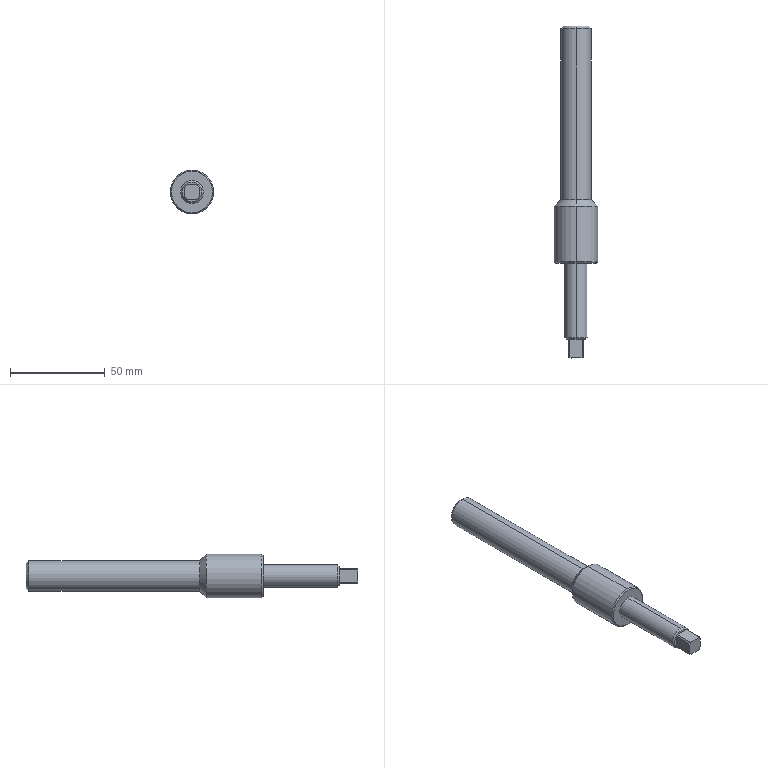Part | SolidWorks | features BaseBody 1 | 1 solid | 33 faces | box 23 x 175 x 23 mm | volume 36998 mm3 | cone 12 | plane 11 | cylinder 10 | commonest cylinder face diameters 10.5 x4 12 x2 16 x2 23 x2
STEP:
#1=CARTESIAN_POINT('',(0.,83.5,8.));
#2=VERTEX_POINT('',#1);
#3=CARTESIAN_POINT('',(0.,83.5,-8.));
#4=VERTEX_POINT('',#3);
#5=CARTESIAN_POINT('',(0.,83.5,0.));
#6=DIRECTION('',(0.,1.,0.));
#7=DIRECTION('',(0.,0.,1.));
#8=AXIS2_PLACEMENT_3D('',#5,#6,#7);
#9=CIRCLE('',#8,8.);
#10=EDGE_CURVE('',#2,#4,#9,.T.);
#11=ORIENTED_EDGE('',*,*,#10,.T.);
#12=CARTESIAN_POINT('',(0.,173.5,-8.));
#13=VERTEX_POINT('',#12);
#14=CARTESIAN_POINT('',(0.,175.,-8.));
#15=DIRECTION('',(0.,1.,0.));
#16=VECTOR('',#15,1000.);
#17=LINE('',#14,#16);
#18=EDGE_CURVE('',#4,#13,#17,.T.);
#19=ORIENTED_EDGE('',*,*,#18,.T.);
#20=CARTESIAN_POINT('',(0.,173.5,8.));
#21=VERTEX_POINT('',#20);
#22=CARTESIAN_POINT('',(0.,173.5,0.));
#23=DIRECTION('',(0.,-1.,0.));
#24=DIRECTION('',(0.,0.,1.));
#25=AXIS2_PLACEMENT_3D('',#22,#23,#24);
#26=CIRCLE('',#25,8.);
#27=EDGE_CURVE('',#13,#21,#26,.T.);
#28=ORIENTED_EDGE('',*,*,#27,.T.);
#29=CARTESIAN_POINT('',(0.,175.,8.));
#30=DIRECTION('',(0.,1.,0.));
#31=VECTOR('',#30,1000.);
#32=LINE('',#29,#31);
#33=EDGE_CURVE('',#2,#21,#32,.T.);
#34=ORIENTED_EDGE('',*,*,#33,.F.);
#35=EDGE_LOOP('',(#11,#19,#28,#34));
#36=FACE_OUTER_BOUND('',#35,.T.);
#37=CARTESIAN_POINT('',(0.,175.,0.));
#38=DIRECTION('',(0.,1.,0.));
#39=DIRECTION('',(0.,0.,1.));
#40=AXIS2_PLACEMENT_3D('',#37,#38,#39);
#41=CYLINDRICAL_SURFACE('',#40,8.);
#42=ADVANCED_FACE('',(#36),#41,.T.);
#43=CARTESIAN_POINT('',(0.,175.,-6.5));
#44=VERTEX_POINT('',#43);
#45=CARTESIAN_POINT('',(0.,175.,6.5));
#46=VERTEX_POINT('',#45);
#47=CARTESIAN_POINT('',(0.,175.,0.));
#48=DIRECTION('',(0.,-1.,0.));
#49=DIRECTION('',(0.,0.,-1.));
#50=AXIS2_PLACEMENT_3D('',#47,#48,#49);
#51=CIRCLE('',#50,6.5);
#52=EDGE_CURVE('',#44,#46,#51,.T.);
#53=ORIENTED_EDGE('',*,*,#52,.T.);
#54=CARTESIAN_POINT('',(0.,173.5,8.));
#55=DIRECTION('',(0.,-0.7071,0.7071));
#56=VECTOR('',#55,1000.);
#57=LINE('',#54,#56);
#58=EDGE_CURVE('',#46,#21,#57,.T.);
#59=ORIENTED_EDGE('',*,*,#58,.T.);
#60=ORIENTED_EDGE('',*,*,#27,.F.);
#61=CARTESIAN_POINT('',(0.,173.5,-8.));
#62=DIRECTION('',(0.,-0.7071,-0.7071));
#63=VECTOR('',#62,1000.);
#64=LINE('',#61,#63);
#65=EDGE_CURVE('',#44,#13,#64,.T.);
#66=ORIENTED_EDGE('',*,*,#65,.F.);
#67=EDGE_LOOP('',(#53,#59,#60,#66));
#68=FACE_OUTER_BOUND('',#67,.T.);
#69=CARTESIAN_POINT('',(0.,173.5,0.));
#70=DIRECTION('',(0.,-1.,0.));
#71=DIRECTION('',(0.,0.,-1.));
#72=AXIS2_PLACEMENT_3D('',#69,#70,#71);
#73=CONICAL_SURFACE('',#72,8.,0.7854);
#74=ADVANCED_FACE('',(#68),#73,.T.);
#75=ORIENTED_EDGE('',*,*,#10,.F.);
#76=CARTESIAN_POINT('',(0.,80.,11.5));
#77=VERTEX_POINT('',#76);
#78=CARTESIAN_POINT('',(0.,80.,11.5));
#79=DIRECTION('',(0.,-0.7071,0.7071));
#80=VECTOR('',#79,1000.);
#81=LINE('',#78,#80);
#82=EDGE_CURVE('',#2,#77,#81,.T.);
#83=ORIENTED_EDGE('',*,*,#82,.T.);
#84=CARTESIAN_POINT('',(0.,80.,-11.5));
#85=VERTEX_POINT('',#84);
#86=CARTESIAN_POINT('',(0.,80.,0.));
#87=DIRECTION('',(0.,1.,0.));
#88=DIRECTION('',(1.,0.,0.));
#89=AXIS2_PLACEMENT_3D('',#86,#87,#88);
#90=CIRCLE('',#89,11.5);
#91=EDGE_CURVE('',#77,#85,#90,.T.);
#92=ORIENTED_EDGE('',*,*,#91,.T.);
#93=CARTESIAN_POINT('',(0.,80.,-11.5));
#94=DIRECTION('',(0.,-0.7071,-0.7071));
#95=VECTOR('',#94,1000.);
#96=LINE('',#93,#95);
#97=EDGE_CURVE('',#4,#85,#96,.T.);
#98=ORIENTED_EDGE('',*,*,#97,.F.);
#99=EDGE_LOOP('',(#75,#83,#92,#98));
#100=FACE_OUTER_BOUND('',#99,.T.);
#101=CARTESIAN_POINT('',(0.,80.,0.));
#102=DIRECTION('',(0.,-1.,0.));
#103=DIRECTION('',(0.,0.,-1.));
#104=AXIS2_PLACEMENT_3D('',#101,#102,#103);
#105=CONICAL_SURFACE('',#104,11.5,0.7854);
#106=ADVANCED_FACE('',(#100),#105,.T.);
#107=CARTESIAN_POINT('',(0.,50.6,11.5));
#108=VERTEX_POINT('',#107);
#109=CARTESIAN_POINT('',(0.,50.6,-11.5));
#110=VERTEX_POINT('',#109);
#111=CARTESIAN_POINT('',(0.,50.6,0.));
#112=DIRECTION('',(0.,1.,0.));
#113=DIRECTION('',(0.,0.,1.));
#114=AXIS2_PLACEMENT_3D('',#111,#112,#113);
#115=CIRCLE('',#114,11.5);
#116=EDGE_CURVE('',#108,#110,#115,.T.);
#117=ORIENTED_EDGE('',*,*,#116,.T.);
#118=CARTESIAN_POINT('',(0.,175.,-11.5));
#119=DIRECTION('',(0.,1.,0.));
#120=VECTOR('',#119,1000.);
#121=LINE('',#118,#120);
#122=EDGE_CURVE('',#110,#85,#121,.T.);
#123=ORIENTED_EDGE('',*,*,#122,.T.);
#124=ORIENTED_EDGE('',*,*,#91,.F.);
#125=CARTESIAN_POINT('',(0.,175.,11.5));
#126=DIRECTION('',(0.,1.,0.));
#127=VECTOR('',#126,1000.);
#128=LINE('',#125,#127);
#129=EDGE_CURVE('',#108,#77,#128,.T.);
#130=ORIENTED_EDGE('',*,*,#129,.F.);
#131=EDGE_LOOP('',(#117,#123,#124,#130));
#132=FACE_OUTER_BOUND('',#131,.T.);
#133=CARTESIAN_POINT('',(0.,175.,0.));
#134=DIRECTION('',(0.,1.,0.));
#135=DIRECTION('',(0.,0.,1.));
#136=AXIS2_PLACEMENT_3D('',#133,#134,#135);
#137=CYLINDRICAL_SURFACE('',#136,11.5);
#138=ADVANCED_FACE('',(#132),#137,.T.);
#139=CARTESIAN_POINT('',(0.,50.,10.9));
#140=VERTEX_POINT('',#139);
#141=CARTESIAN_POINT('',(0.,50.,-10.9));
#142=VERTEX_POINT('',#141);
#143=CARTESIAN_POINT('',(0.,50.,0.));
#144=DIRECTION('',(0.,1.,0.));
#145=DIRECTION('',(0.,0.,1.));
#146=AXIS2_PLACEMENT_3D('',#143,#144,#145);
#147=CIRCLE('',#146,10.9);
#148=EDGE_CURVE('',#140,#142,#147,.T.);
#149=ORIENTED_EDGE('',*,*,#148,.T.);
#150=CARTESIAN_POINT('',(0.,50.6,-11.5));
#151=DIRECTION('',(0.,0.7071,-0.7071));
#152=VECTOR('',#151,1000.);
#153=LINE('',#150,#152);
#154=EDGE_CURVE('',#142,#110,#153,.T.);
#155=ORIENTED_EDGE('',*,*,#154,.T.);
#156=ORIENTED_EDGE('',*,*,#116,.F.);
#157=CARTESIAN_POINT('',(0.,50.6,11.5));
#158=DIRECTION('',(0.,0.7071,0.7071));
#159=VECTOR('',#158,1000.);
#160=LINE('',#157,#159);
#161=EDGE_CURVE('',#140,#108,#160,.T.);
#162=ORIENTED_EDGE('',*,*,#161,.F.);
#163=EDGE_LOOP('',(#149,#155,#156,#162));
#164=FACE_OUTER_BOUND('',#163,.T.);
#165=CARTESIAN_POINT('',(0.,50.6,0.));
#166=DIRECTION('',(0.,1.,0.));
#167=DIRECTION('',(0.,0.,1.));
#168=AXIS2_PLACEMENT_3D('',#165,#166,#167);
#169=CONICAL_SURFACE('',#168,11.5,0.7854);
#170=ADVANCED_FACE('',(#164),#169,.T.);
#171=CARTESIAN_POINT('',(0.,10.75,6.));
#172=VERTEX_POINT('',#171);
#173=CARTESIAN_POINT('',(0.,10.75,-6.));
#174=VERTEX_POINT('',#173);
#175=CARTESIAN_POINT('',(0.,10.75,0.));
#176=DIRECTION('',(0.,1.,0.));
#177=DIRECTION('',(0.,0.,1.));
#178=AXIS2_PLACEMENT_3D('',#175,#176,#177);
#179=CIRCLE('',#178,6.);
#180=EDGE_CURVE('',#172,#174,#179,.T.);
#181=ORIENTED_EDGE('',*,*,#180,.T.);
#182=CARTESIAN_POINT('',(0.,50.,-6.));
#183=VERTEX_POINT('',#182);
#184=CARTESIAN_POINT('',(0.,175.,-6.));
#185=DIRECTION('',(0.,1.,0.));
#186=VECTOR('',#185,1000.);
#187=LINE('',#184,#186);
#188=EDGE_CURVE('',#174,#183,#187,.T.);
#189=ORIENTED_EDGE('',*,*,#188,.T.);
#190=CARTESIAN_POINT('',(0.,50.,6.));
#191=VERTEX_POINT('',#190);
#192=CARTESIAN_POINT('',(0.,50.,0.));
#193=DIRECTION('',(0.,1.,0.));
#194=DIRECTION('',(0.,0.,1.));
#195=AXIS2_PLACEMENT_3D('',#192,#193,#194);
#196=CIRCLE('',#195,6.);
#197=EDGE_CURVE('',#191,#183,#196,.T.);
#198=ORIENTED_EDGE('',*,*,#197,.F.);
#199=CARTESIAN_POINT('',(0.,175.,6.));
#200=DIRECTION('',(0.,1.,0.));
#201=VECTOR('',#200,1000.);
#202=LINE('',#199,#201);
#203=EDGE_CURVE('',#172,#191,#202,.T.);
#204=ORIENTED_EDGE('',*,*,#203,.F.);
#205=EDGE_LOOP('',(#181,#189,#198,#204));
#206=FACE_OUTER_BOUND('',#205,.T.);
#207=CARTESIAN_POINT('',(0.,175.,0.));
#208=DIRECTION('',(0.,1.,0.));
#209=DIRECTION('',(0.,0.,1.));
#210=AXIS2_PLACEMENT_3D('',#207,#208,#209);
#211=CYLINDRICAL_SURFACE('',#210,6.);
#212=ADVANCED_FACE('',(#206),#211,.T.);
#213=CARTESIAN_POINT('',(3.4,10.,-4.));
#214=VERTEX_POINT('',#213);
#215=CARTESIAN_POINT('',(0.,10.,-5.25));
#216=VERTEX_POINT('',#215);
#217=CARTESIAN_POINT('',(0.,10.,0.));
#218=DIRECTION('',(0.,1.,0.));
#219=DIRECTION('',(0.,0.,1.));
#220=AXIS2_PLACEMENT_3D('',#217,#218,#219);
#221=CIRCLE('',#220,5.25);
#222=EDGE_CURVE('',#214,#216,#221,.T.);
#223=ORIENTED_EDGE('',*,*,#222,.T.);
#224=CARTESIAN_POINT('',(0.,10.75,-6.));
#225=DIRECTION('',(0.,0.7071,-0.7071));
#226=VECTOR('',#225,1000.);
#227=LINE('',#224,#226);
#228=EDGE_CURVE('',#216,#174,#227,.T.);
#229=ORIENTED_EDGE('',*,*,#228,.T.);
#230=ORIENTED_EDGE('',*,*,#180,.F.);
#231=CARTESIAN_POINT('',(0.,10.,5.25));
#232=VERTEX_POINT('',#231);
#233=CARTESIAN_POINT('',(0.,10.75,6.));
#234=DIRECTION('',(0.,0.7071,0.7071));
#235=VECTOR('',#234,1000.);
#236=LINE('',#233,#235);
#237=EDGE_CURVE('',#232,#172,#236,.T.);
#238=ORIENTED_EDGE('',*,*,#237,.F.);
#239=CARTESIAN_POINT('',(3.4,10.,4.));
#240=VERTEX_POINT('',#239);
#241=CARTESIAN_POINT('',(0.,10.,0.));
#242=DIRECTION('',(0.,1.,0.));
#243=DIRECTION('',(0.,0.,1.));
#244=AXIS2_PLACEMENT_3D('',#241,#242,#243);
#245=CIRCLE('',#244,5.25);
#246=EDGE_CURVE('',#232,#240,#245,.T.);
#247=ORIENTED_EDGE('',*,*,#246,.T.);
#248=CARTESIAN_POINT('',(4.,10.,3.4));
#249=VERTEX_POINT('',#248);
#250=CARTESIAN_POINT('',(0.,10.,0.));
#251=DIRECTION('',(0.,-1.,0.));
#252=DIRECTION('',(0.,0.,1.));
#253=AXIS2_PLACEMENT_3D('',#250,#251,#252);
#254=CIRCLE('',#253,5.25);
#255=EDGE_CURVE('',#249,#240,#254,.T.);
#256=ORIENTED_EDGE('',*,*,#255,.F.);
#257=CARTESIAN_POINT('',(4.,10.,-3.4));
#258=VERTEX_POINT('',#257);
#259=CARTESIAN_POINT('',(0.,10.,0.));
#260=DIRECTION('',(0.,1.,0.));
#261=DIRECTION('',(0.,0.,1.));
#262=AXIS2_PLACEMENT_3D('',#259,#260,#261);
#263=CIRCLE('',#262,5.25);
#264=EDGE_CURVE('',#249,#258,#263,.T.);
#265=ORIENTED_EDGE('',*,*,#264,.T.);
#266=CARTESIAN_POINT('',(0.,10.,0.));
#267=DIRECTION('',(0.,-1.,0.));
#268=DIRECTION('',(0.,0.,1.));
#269=AXIS2_PLACEMENT_3D('',#266,#267,#268);
#270=CIRCLE('',#269,5.25);
#271=EDGE_CURVE('',#214,#258,#270,.T.);
#272=ORIENTED_EDGE('',*,*,#271,.F.);
#273=EDGE_LOOP('',(#223,#229,#230,#238,#247,#256,#265,#272));
#274=FACE_OUTER_BOUND('',#273,.T.);
#275=CARTESIAN_POINT('',(0.,10.75,0.));
#276=DIRECTION('',(0.,1.,0.));
#277=DIRECTION('',(0.,0.,1.));
#278=AXIS2_PLACEMENT_3D('',#275,#276,#277);
#279=CONICAL_SURFACE('',#278,6.,0.7854);
#280=ADVANCED_FACE('',(#274),#279,.T.);
#281=ORIENTED_EDGE('',*,*,#18,.F.);
#282=CARTESIAN_POINT('',(0.,83.5,0.));
#283=DIRECTION('',(0.,1.,0.));
#284=DIRECTION('',(0.,0.,1.));
#285=AXIS2_PLACEMENT_3D('',#282,#283,#284);
#286=CIRCLE('',#285,8.);
#287=EDGE_CURVE('',#4,#2,#286,.T.);
#288=ORIENTED_EDGE('',*,*,#287,.T.);
#289=ORIENTED_EDGE('',*,*,#33,.T.);
#290=CARTESIAN_POINT('',(0.,173.5,0.));
#291=DIRECTION('',(0.,-1.,0.));
#292=DIRECTION('',(0.,0.,1.));
#293=AXIS2_PLACEMENT_3D('',#290,#291,#292);
#294=CIRCLE('',#293,8.);
#295=EDGE_CURVE('',#21,#13,#294,.T.);
#296=ORIENTED_EDGE('',*,*,#295,.T.);
#297=EDGE_LOOP('',(#281,#288,#289,#296));
#298=FACE_OUTER_BOUND('',#297,.T.);
#299=CARTESIAN_POINT('',(0.,175.,0.));
#300=DIRECTION('',(0.,1.,0.));
#301=DIRECTION('',(0.,0.,1.));
#302=AXIS2_PLACEMENT_3D('',#299,#300,#301);
#303=CYLINDRICAL_SURFACE('',#302,8.);
#304=ADVANCED_FACE('',(#298),#303,.T.);
#305=ORIENTED_EDGE('',*,*,#58,.F.);
#306=CARTESIAN_POINT('',(0.,175.,0.));
#307=DIRECTION('',(0.,-1.,0.));
#308=DIRECTION('',(0.,0.,-1.));
#309=AXIS2_PLACEMENT_3D('',#306,#307,#308);
#310=CIRCLE('',#309,6.5);
#311=EDGE_CURVE('',#46,#44,#310,.T.);
#312=ORIENTED_EDGE('',*,*,#311,.T.);
#313=ORIENTED_EDGE('',*,*,#65,.T.);
#314=ORIENTED_EDGE('',*,*,#295,.F.);
#315=EDGE_LOOP('',(#305,#312,#313,#314));
#316=FACE_OUTER_BOUND('',#315,.T.);
#317=CARTESIAN_POINT('',(0.,173.5,0.));
#318=DIRECTION('',(0.,-1.,0.));
#319=DIRECTION('',(0.,0.,-1.));
#320=AXIS2_PLACEMENT_3D('',#317,#318,#319);
#321=CONICAL_SURFACE('',#320,8.,0.7854);
#322=ADVANCED_FACE('',(#316),#321,.T.);
#323=ORIENTED_EDGE('',*,*,#82,.F.);
#324=ORIENTED_EDGE('',*,*,#287,.F.);
#325=ORIENTED_EDGE('',*,*,#97,.T.);
#326=CARTESIAN_POINT('',(0.,80.,0.));
#327=DIRECTION('',(0.,1.,0.));
#328=DIRECTION('',(1.,0.,0.));
#329=AXIS2_PLACEMENT_3D('',#326,#327,#328);
#330=CIRCLE('',#329,11.5);
#331=EDGE_CURVE('',#85,#77,#330,.T.);
#332=ORIENTED_EDGE('',*,*,#331,.T.);
#333=EDGE_LOOP('',(#323,#324,#325,#332));
#334=FACE_OUTER_BOUND('',#333,.T.);
#335=CARTESIAN_POINT('',(0.,80.,0.));
#336=DIRECTION('',(0.,-1.,0.));
#337=DIRECTION('',(0.,0.,-1.));
#338=AXIS2_PLACEMENT_3D('',#335,#336,#337);
#339=CONICAL_SURFACE('',#338,11.5,0.7854);
#340=ADVANCED_FACE('',(#334),#339,.T.);
#341=ORIENTED_EDGE('',*,*,#52,.F.);
#342=ORIENTED_EDGE('',*,*,#311,.F.);
#343=EDGE_LOOP('',(#341,#342));
#344=FACE_OUTER_BOUND('',#343,.T.);
#345=CARTESIAN_POINT('',(-6.5,175.,0.));
#346=DIRECTION('',(0.,1.,0.));
#347=DIRECTION('',(-1.,0.,0.));
#348=AXIS2_PLACEMENT_3D('',#345,#346,#347);
#349=PLANE('',#348);
#350=ADVANCED_FACE('',(#344),#349,.T.);
#351=ORIENTED_EDGE('',*,*,#122,.F.);
#352=CARTESIAN_POINT('',(0.,50.6,0.));
#353=DIRECTION('',(0.,1.,0.));
#354=DIRECTION('',(0.,0.,1.));
#355=AXIS2_PLACEMENT_3D('',#352,#353,#354);
#356=CIRCLE('',#355,11.5);
#357=EDGE_CURVE('',#110,#108,#356,.T.);
#358=ORIENTED_EDGE('',*,*,#357,.T.);
#359=ORIENTED_EDGE('',*,*,#129,.T.);
#360=ORIENTED_EDGE('',*,*,#331,.F.);
#361=EDGE_LOOP('',(#351,#358,#359,#360));
#362=FACE_OUTER_BOUND('',#361,.T.);
#363=CARTESIAN_POINT('',(0.,175.,0.));
#364=DIRECTION('',(0.,1.,0.));
#365=DIRECTION('',(0.,0.,1.));
#366=AXIS2_PLACEMENT_3D('',#363,#364,#365);
#367=CYLINDRICAL_SURFACE('',#366,11.5);
#368=ADVANCED_FACE('',(#362),#367,.T.);
#369=ORIENTED_EDGE('',*,*,#154,.F.);
#370=CARTESIAN_POINT('',(0.,50.,0.));
#371=DIRECTION('',(0.,1.,0.));
#372=DIRECTION('',(0.,0.,1.));
#373=AXIS2_PLACEMENT_3D('',#370,#371,#372);
#374=CIRCLE('',#373,10.9);
#375=EDGE_CURVE('',#142,#140,#374,.T.);
#376=ORIENTED_EDGE('',*,*,#375,.T.);
#377=ORIENTED_EDGE('',*,*,#161,.T.);
#378=ORIENTED_EDGE('',*,*,#357,.F.);
#379=EDGE_LOOP('',(#369,#376,#377,#378));
#380=FACE_OUTER_BOUND('',#379,.T.);
#381=CARTESIAN_POINT('',(0.,50.6,0.));
#382=DIRECTION('',(0.,1.,0.));
#383=DIRECTION('',(0.,0.,1.));
#384=AXIS2_PLACEMENT_3D('',#381,#382,#383);
#385=CONICAL_SURFACE('',#384,11.5,0.7854);
#386=ADVANCED_FACE('',(#380),#385,.T.);
#387=ORIENTED_EDGE('',*,*,#197,.T.);
#388=CARTESIAN_POINT('',(0.,50.,0.));
#389=DIRECTION('',(0.,1.,0.));
#390=DIRECTION('',(0.,0.,1.));
#391=AXIS2_PLACEMENT_3D('',#388,#389,#390);
#392=CIRCLE('',#391,6.);
#393=EDGE_CURVE('',#183,#191,#392,.T.);
#394=ORIENTED_EDGE('',*,*,#393,.T.);
#395=EDGE_LOOP('',(#387,#394));
#396=FACE_BOUND('',#395,.T.);
#397=ORIENTED_EDGE('',*,*,#148,.F.);
#398=ORIENTED_EDGE('',*,*,#375,.F.);
#399=EDGE_LOOP('',(#397,#398));
#400=FACE_OUTER_BOUND('',#399,.T.);
#401=CARTESIAN_POINT('',(-6.,50.,0.));
#402=DIRECTION('',(0.,-1.,0.));
#403=DIRECTION('',(1.,0.,0.));
#404=AXIS2_PLACEMENT_3D('',#401,#402,#403);
#405=PLANE('',#404);
#406=ADVANCED_FACE('',(#396,#400),#405,.T.);
#407=ORIENTED_EDGE('',*,*,#188,.F.);
#408=CARTESIAN_POINT('',(0.,10.75,0.));
#409=DIRECTION('',(0.,1.,0.));
#410=DIRECTION('',(0.,0.,1.));
#411=AXIS2_PLACEMENT_3D('',#408,#409,#410);
#412=CIRCLE('',#411,6.);
#413=EDGE_CURVE('',#174,#172,#412,.T.);
#414=ORIENTED_EDGE('',*,*,#413,.T.);
#415=ORIENTED_EDGE('',*,*,#203,.T.);
#416=ORIENTED_EDGE('',*,*,#393,.F.);
#417=EDGE_LOOP('',(#407,#414,#415,#416));
#418=FACE_OUTER_BOUND('',#417,.T.);
#419=CARTESIAN_POINT('',(0.,175.,0.));
#420=DIRECTION('',(0.,1.,0.));
#421=DIRECTION('',(0.,0.,1.));
#422=AXIS2_PLACEMENT_3D('',#419,#420,#421);
#423=CYLINDRICAL_SURFACE('',#422,6.);
#424=ADVANCED_FACE('',(#418),#423,.T.);
#425=ORIENTED_EDGE('',*,*,#228,.F.);
#426=CARTESIAN_POINT('',(-3.4,10.,-4.));
#427=VERTEX_POINT('',#426);
#428=CARTESIAN_POINT('',(0.,10.,0.));
#429=DIRECTION('',(0.,1.,0.));
#430=DIRECTION('',(0.,0.,1.));
#431=AXIS2_PLACEMENT_3D('',#428,#429,#430);
#432=CIRCLE('',#431,5.25);
#433=EDGE_CURVE('',#216,#427,#432,.T.);
#434=ORIENTED_EDGE('',*,*,#433,.T.);
#435=CARTESIAN_POINT('',(-4.,10.,-3.4));
#436=VERTEX_POINT('',#435);
#437=CARTESIAN_POINT('',(0.,10.,0.));
#438=DIRECTION('',(0.,-1.,0.));
#439=DIRECTION('',(0.,0.,1.));
#440=AXIS2_PLACEMENT_3D('',#437,#438,#439);
#441=CIRCLE('',#440,5.25);
#442=EDGE_CURVE('',#436,#427,#441,.T.);
#443=ORIENTED_EDGE('',*,*,#442,.F.);
#444=CARTESIAN_POINT('',(-4.,10.,3.4));
#445=VERTEX_POINT('',#444);
#446=CARTESIAN_POINT('',(0.,10.,0.));
#447=DIRECTION('',(0.,1.,0.));
#448=DIRECTION('',(0.,0.,1.));
#449=AXIS2_PLACEMENT_3D('',#446,#447,#448);
#450=CIRCLE('',#449,5.25);
#451=EDGE_CURVE('',#436,#445,#450,.T.);
#452=ORIENTED_EDGE('',*,*,#451,.T.);
#453=CARTESIAN_POINT('',(-3.4,10.,4.));
#454=VERTEX_POINT('',#453);
#455=CARTESIAN_POINT('',(0.,10.,0.));
#456=DIRECTION('',(0.,-1.,0.));
#457=DIRECTION('',(0.,0.,1.));
#458=AXIS2_PLACEMENT_3D('',#455,#456,#457);
#459=CIRCLE('',#458,5.25);
#460=EDGE_CURVE('',#454,#445,#459,.T.);
#461=ORIENTED_EDGE('',*,*,#460,.F.);
#462=CARTESIAN_POINT('',(0.,10.,0.));
#463=DIRECTION('',(0.,1.,0.));
#464=DIRECTION('',(0.,0.,1.));
#465=AXIS2_PLACEMENT_3D('',#462,#463,#464);
#466=CIRCLE('',#465,5.25);
#467=EDGE_CURVE('',#454,#232,#466,.T.);
#468=ORIENTED_EDGE('',*,*,#467,.T.);
#469=ORIENTED_EDGE('',*,*,#237,.T.);
#470=ORIENTED_EDGE('',*,*,#413,.F.);
#471=EDGE_LOOP('',(#425,#434,#443,#452,#461,#468,#469,#470));
#472=FACE_OUTER_BOUND('',#471,.T.);
#473=CARTESIAN_POINT('',(0.,10.75,0.));
#474=DIRECTION('',(0.,1.,0.));
#475=DIRECTION('',(0.,0.,1.));
#476=AXIS2_PLACEMENT_3D('',#473,#474,#475);
#477=CONICAL_SURFACE('',#476,6.,0.7854);
#478=ADVANCED_FACE('',(#472),#477,.T.);
#479=CARTESIAN_POINT('',(-4.,10.,0.));
#480=DIRECTION('',(0.,0.,1.));
#481=VECTOR('',#480,1000.);
#482=LINE('',#479,#481);
#483=EDGE_CURVE('',#436,#445,#482,.T.);
#484=ORIENTED_EDGE('',*,*,#483,.T.);
#485=ORIENTED_EDGE('',*,*,#451,.F.);
#486=EDGE_LOOP('',(#484,#485));
#487=FACE_OUTER_BOUND('',#486,.T.);
#488=CARTESIAN_POINT('',(0.,10.,0.));
#489=DIRECTION('',(0.,-1.,0.));
#490=DIRECTION('',(1.,0.,0.));
#491=AXIS2_PLACEMENT_3D('',#488,#489,#490);
#492=PLANE('',#491);
#493=ADVANCED_FACE('',(#487),#492,.T.);
#494=CARTESIAN_POINT('',(0.,10.,-4.));
#495=DIRECTION('',(-1.,0.,0.));
#496=VECTOR('',#495,1000.);
#497=LINE('',#494,#496);
#498=EDGE_CURVE('',#214,#427,#497,.T.);
#499=ORIENTED_EDGE('',*,*,#498,.T.);
#500=ORIENTED_EDGE('',*,*,#433,.F.);
#501=ORIENTED_EDGE('',*,*,#222,.F.);
#502=EDGE_LOOP('',(#499,#500,#501));
#503=FACE_OUTER_BOUND('',#502,.T.);
#504=CARTESIAN_POINT('',(0.,10.,0.));
#505=DIRECTION('',(0.,-1.,0.));
#506=DIRECTION('',(1.,0.,0.));
#507=AXIS2_PLACEMENT_3D('',#504,#505,#506);
#508=PLANE('',#507);
#509=ADVANCED_FACE('',(#503),#508,.T.);
#510=ORIENTED_EDGE('',*,*,#264,.F.);
#511=CARTESIAN_POINT('',(4.,10.,0.));
#512=DIRECTION('',(0.,0.,-1.));
#513=VECTOR('',#512,1000.);
#514=LINE('',#511,#513);
#515=EDGE_CURVE('',#249,#258,#514,.T.);
#516=ORIENTED_EDGE('',*,*,#515,.T.);
#517=EDGE_LOOP('',(#510,#516));
#518=FACE_OUTER_BOUND('',#517,.T.);
#519=CARTESIAN_POINT('',(0.,10.,0.));
#520=DIRECTION('',(0.,-1.,0.));
#521=DIRECTION('',(1.,0.,0.));
#522=AXIS2_PLACEMENT_3D('',#519,#520,#521);
#523=PLANE('',#522);
#524=ADVANCED_FACE('',(#518),#523,.T.);
#525=CARTESIAN_POINT('',(0.,10.,4.));
#526=DIRECTION('',(1.,0.,0.));
#527=VECTOR('',#526,1000.);
#528=LINE('',#525,#527);
#529=EDGE_CURVE('',#454,#240,#528,.T.);
#530=ORIENTED_EDGE('',*,*,#529,.T.);
#531=ORIENTED_EDGE('',*,*,#246,.F.);
#532=ORIENTED_EDGE('',*,*,#467,.F.);
#533=EDGE_LOOP('',(#530,#531,#532));
#534=FACE_OUTER_BOUND('',#533,.T.);
#535=CARTESIAN_POINT('',(0.,10.,0.));
#536=DIRECTION('',(0.,-1.,0.));
#537=DIRECTION('',(1.,0.,0.));
#538=AXIS2_PLACEMENT_3D('',#535,#536,#537);
#539=PLANE('',#538);
#540=ADVANCED_FACE('',(#534),#539,.T.);
#541=CARTESIAN_POINT('',(-4.,0.,-2.562));
#542=VERTEX_POINT('',#541);
#543=CARTESIAN_POINT('',(-4.,0.,2.562));
#544=VERTEX_POINT('',#543);
#545=CARTESIAN_POINT('',(-4.,0.,-4.));
#546=DIRECTION('',(0.,0.,1.));
#547=VECTOR('',#546,1000.);
#548=LINE('',#545,#547);
#549=EDGE_CURVE('',#542,#544,#548,.T.);
#550=ORIENTED_EDGE('',*,*,#549,.T.);
#551=CARTESIAN_POINT('',(-4.,0.5,3.4));
#552=VERTEX_POINT('',#551);
#553=CARTESIAN_POINT('',(-4.,0.5,3.4));
#554=CARTESIAN_POINT('',(-4.,0.323,3.127));
#555=CARTESIAN_POINT('',(-4.,0.1546,2.848));
#556=CARTESIAN_POINT('',(-4.,0.,2.562));
#557=B_SPLINE_CURVE_WITH_KNOTS('',3,(#553,#554,#555,#556),.UNSPECIFIED.,.F.,.F.,(4,4),(0.,0.0009764),.UNSPECIFIED.);
#558=EDGE_CURVE('',#552,#544,#557,.T.);
#559=ORIENTED_EDGE('',*,*,#558,.F.);
#560=CARTESIAN_POINT('',(-4.,10.,3.4));
#561=DIRECTION('',(0.,1.,0.));
#562=VECTOR('',#561,1000.);
#563=LINE('',#560,#562);
#564=EDGE_CURVE('',#552,#445,#563,.T.);
#565=ORIENTED_EDGE('',*,*,#564,.T.);
#566=ORIENTED_EDGE('',*,*,#483,.F.);
#567=CARTESIAN_POINT('',(-4.,0.5,-3.4));
#568=VERTEX_POINT('',#567);
#569=CARTESIAN_POINT('',(-4.,10.,-3.4));
#570=DIRECTION('',(0.,-1.,0.));
#571=VECTOR('',#570,1000.);
#572=LINE('',#569,#571);
#573=EDGE_CURVE('',#436,#568,#572,.T.);
#574=ORIENTED_EDGE('',*,*,#573,.T.);
#575=CARTESIAN_POINT('',(-4.,0.,-2.562));
#576=CARTESIAN_POINT('',(-4.,0.1546,-2.848));
#577=CARTESIAN_POINT('',(-4.,0.323,-3.127));
#578=CARTESIAN_POINT('',(-4.,0.5,-3.4));
#579=B_SPLINE_CURVE_WITH_KNOTS('',3,(#575,#576,#577,#578),.UNSPECIFIED.,.F.,.F.,(4,4),(0.,0.0009764),.UNSPECIFIED.);
#580=EDGE_CURVE('',#542,#568,#579,.T.);
#581=ORIENTED_EDGE('',*,*,#580,.F.);
#582=EDGE_LOOP('',(#550,#559,#565,#566,#574,#581));
#583=FACE_OUTER_BOUND('',#582,.T.);
#584=CARTESIAN_POINT('',(-4.,10.,-4.));
#585=DIRECTION('',(-1.,0.,0.));
#586=DIRECTION('',(0.,-1.,0.));
#587=AXIS2_PLACEMENT_3D('',#584,#585,#586);
#588=PLANE('',#587);
#589=ADVANCED_FACE('',(#583),#588,.T.);
#590=CARTESIAN_POINT('',(2.562,0.,-4.));
#591=VERTEX_POINT('',#590);
#592=CARTESIAN_POINT('',(-2.562,0.,-4.));
#593=VERTEX_POINT('',#592);
#594=CARTESIAN_POINT('',(4.,0.,-4.));
#595=DIRECTION('',(-1.,0.,0.));
#596=VECTOR('',#595,1000.);
#597=LINE('',#594,#596);
#598=EDGE_CURVE('',#591,#593,#597,.T.);
#599=ORIENTED_EDGE('',*,*,#598,.T.);
#600=CARTESIAN_POINT('',(-3.4,0.5,-4.));
#601=VERTEX_POINT('',#600);
#602=CARTESIAN_POINT('',(-3.4,0.5,-4.));
#603=CARTESIAN_POINT('',(-3.127,0.323,-4.));
#604=CARTESIAN_POINT('',(-2.848,0.1546,-4.));
#605=CARTESIAN_POINT('',(-2.562,0.,-4.));
#606=B_SPLINE_CURVE_WITH_KNOTS('',3,(#602,#603,#604,#605),.UNSPECIFIED.,.F.,.F.,(4,4),(0.,0.0009764),.UNSPECIFIED.);
#607=EDGE_CURVE('',#601,#593,#606,.T.);
#608=ORIENTED_EDGE('',*,*,#607,.F.);
#609=CARTESIAN_POINT('',(-3.4,10.,-4.));
#610=DIRECTION('',(0.,1.,0.));
#611=VECTOR('',#610,1000.);
#612=LINE('',#609,#611);
#613=EDGE_CURVE('',#601,#427,#612,.T.);
#614=ORIENTED_EDGE('',*,*,#613,.T.);
#615=ORIENTED_EDGE('',*,*,#498,.F.);
#616=CARTESIAN_POINT('',(3.4,0.5,-4.));
#617=VERTEX_POINT('',#616);
#618=CARTESIAN_POINT('',(3.4,10.,-4.));
#619=DIRECTION('',(0.,-1.,0.));
#620=VECTOR('',#619,1000.);
#621=LINE('',#618,#620);
#622=EDGE_CURVE('',#214,#617,#621,.T.);
#623=ORIENTED_EDGE('',*,*,#622,.T.);
#624=CARTESIAN_POINT('',(2.562,0.,-4.));
#625=CARTESIAN_POINT('',(2.848,0.1546,-4.));
#626=CARTESIAN_POINT('',(3.127,0.323,-4.));
#627=CARTESIAN_POINT('',(3.4,0.5,-4.));
#628=B_SPLINE_CURVE_WITH_KNOTS('',3,(#624,#625,#626,#627),.UNSPECIFIED.,.F.,.F.,(4,4),(0.,0.0009764),.UNSPECIFIED.);
#629=EDGE_CURVE('',#591,#617,#628,.T.);
#630=ORIENTED_EDGE('',*,*,#629,.F.);
#631=EDGE_LOOP('',(#599,#608,#614,#615,#623,#630));
#632=FACE_OUTER_BOUND('',#631,.T.);
#633=CARTESIAN_POINT('',(4.,10.,-4.));
#634=DIRECTION('',(0.,0.,-1.));
#635=DIRECTION('',(-1.,0.,0.));
#636=AXIS2_PLACEMENT_3D('',#633,#634,#635);
#637=PLANE('',#636);
#638=ADVANCED_FACE('',(#632),#637,.T.);
#639=CARTESIAN_POINT('',(4.,0.,2.562));
#640=VERTEX_POINT('',#639);
#641=CARTESIAN_POINT('',(4.,0.,-2.562));
#642=VERTEX_POINT('',#641);
#643=CARTESIAN_POINT('',(4.,0.,-4.));
#644=DIRECTION('',(0.,0.,-1.));
#645=VECTOR('',#644,1000.);
#646=LINE('',#643,#645);
#647=EDGE_CURVE('',#640,#642,#646,.T.);
#648=ORIENTED_EDGE('',*,*,#647,.T.);
#649=CARTESIAN_POINT('',(4.,0.5,-3.4));
#650=VERTEX_POINT('',#649);
#651=CARTESIAN_POINT('',(4.,0.5,-3.4));
#652=CARTESIAN_POINT('',(4.,0.323,-3.127));
#653=CARTESIAN_POINT('',(4.,0.1546,-2.848));
#654=CARTESIAN_POINT('',(4.,0.,-2.562));
#655=B_SPLINE_CURVE_WITH_KNOTS('',3,(#651,#652,#653,#654),.UNSPECIFIED.,.F.,.F.,(4,4),(0.,0.0009764),.UNSPECIFIED.);
#656=EDGE_CURVE('',#650,#642,#655,.T.);
#657=ORIENTED_EDGE('',*,*,#656,.F.);
#658=CARTESIAN_POINT('',(4.,10.,-3.4));
#659=DIRECTION('',(0.,1.,0.));
#660=VECTOR('',#659,1000.);
#661=LINE('',#658,#660);
#662=EDGE_CURVE('',#650,#258,#661,.T.);
#663=ORIENTED_EDGE('',*,*,#662,.T.);
#664=ORIENTED_EDGE('',*,*,#515,.F.);
#665=CARTESIAN_POINT('',(4.,0.5,3.4));
#666=VERTEX_POINT('',#665);
#667=CARTESIAN_POINT('',(4.,10.,3.4));
#668=DIRECTION('',(0.,-1.,0.));
#669=VECTOR('',#668,1000.);
#670=LINE('',#667,#669);
#671=EDGE_CURVE('',#249,#666,#670,.T.);
#672=ORIENTED_EDGE('',*,*,#671,.T.);
#673=CARTESIAN_POINT('',(4.,0.,2.562));
#674=CARTESIAN_POINT('',(4.,0.1546,2.848));
#675=CARTESIAN_POINT('',(4.,0.323,3.127));
#676=CARTESIAN_POINT('',(4.,0.5,3.4));
#677=B_SPLINE_CURVE_WITH_KNOTS('',3,(#673,#674,#675,#676),.UNSPECIFIED.,.F.,.F.,(4,4),(0.,0.0009764),.UNSPECIFIED.);
#678=EDGE_CURVE('',#640,#666,#677,.T.);
#679=ORIENTED_EDGE('',*,*,#678,.F.);
#680=EDGE_LOOP('',(#648,#657,#663,#664,#672,#679));
#681=FACE_OUTER_BOUND('',#680,.T.);
#682=CARTESIAN_POINT('',(4.,10.,-4.));
#683=DIRECTION('',(1.,0.,0.));
#684=DIRECTION('',(0.,1.,0.));
#685=AXIS2_PLACEMENT_3D('',#682,#683,#684);
#686=PLANE('',#685);
#687=ADVANCED_FACE('',(#681),#686,.T.);
#688=CARTESIAN_POINT('',(-2.562,0.,4.));
#689=VERTEX_POINT('',#688);
#690=CARTESIAN_POINT('',(2.562,0.,4.));
#691=VERTEX_POINT('',#690);
#692=CARTESIAN_POINT('',(4.,0.,4.));
#693=DIRECTION('',(1.,0.,0.));
#694=VECTOR('',#693,1000.);
#695=LINE('',#692,#694);
#696=EDGE_CURVE('',#689,#691,#695,.T.);
#697=ORIENTED_EDGE('',*,*,#696,.T.);
#698=CARTESIAN_POINT('',(3.4,0.5,4.));
#699=VERTEX_POINT('',#698);
#700=CARTESIAN_POINT('',(3.4,0.5,4.));
#701=CARTESIAN_POINT('',(3.127,0.323,4.));
#702=CARTESIAN_POINT('',(2.848,0.1546,4.));
#703=CARTESIAN_POINT('',(2.562,0.,4.));
#704=B_SPLINE_CURVE_WITH_KNOTS('',3,(#700,#701,#702,#703),.UNSPECIFIED.,.F.,.F.,(4,4),(0.,0.0009764),.UNSPECIFIED.);
#705=EDGE_CURVE('',#699,#691,#704,.T.);
#706=ORIENTED_EDGE('',*,*,#705,.F.);
#707=CARTESIAN_POINT('',(3.4,10.,4.));
#708=DIRECTION('',(0.,1.,0.));
#709=VECTOR('',#708,1000.);
#710=LINE('',#707,#709);
#711=EDGE_CURVE('',#699,#240,#710,.T.);
#712=ORIENTED_EDGE('',*,*,#711,.T.);
#713=ORIENTED_EDGE('',*,*,#529,.F.);
#714=CARTESIAN_POINT('',(-3.4,0.5,4.));
#715=VERTEX_POINT('',#714);
#716=CARTESIAN_POINT('',(-3.4,10.,4.));
#717=DIRECTION('',(0.,-1.,0.));
#718=VECTOR('',#717,1000.);
#719=LINE('',#716,#718);
#720=EDGE_CURVE('',#454,#715,#719,.T.);
#721=ORIENTED_EDGE('',*,*,#720,.T.);
#722=CARTESIAN_POINT('',(-2.562,0.,4.));
#723=CARTESIAN_POINT('',(-2.848,0.1546,4.));
#724=CARTESIAN_POINT('',(-3.127,0.323,4.));
#725=CARTESIAN_POINT('',(-3.4,0.5,4.));
#726=B_SPLINE_CURVE_WITH_KNOTS('',3,(#722,#723,#724,#725),.UNSPECIFIED.,.F.,.F.,(4,4),(0.,0.0009764),.UNSPECIFIED.);
#727=EDGE_CURVE('',#689,#715,#726,.T.);
#728=ORIENTED_EDGE('',*,*,#727,.F.);
#729=EDGE_LOOP('',(#697,#706,#712,#713,#721,#728));
#730=FACE_OUTER_BOUND('',#729,.T.);
#731=CARTESIAN_POINT('',(4.,10.,4.));
#732=DIRECTION('',(0.,0.,1.));
#733=DIRECTION('',(1.,0.,0.));
#734=AXIS2_PLACEMENT_3D('',#731,#732,#733);
#735=PLANE('',#734);
#736=ADVANCED_FACE('',(#730),#735,.T.);
#737=CARTESIAN_POINT('',(0.,0.,0.));
#738=DIRECTION('',(0.,-1.,0.));
#739=DIRECTION('',(-1.,0.,0.));
#740=AXIS2_PLACEMENT_3D('',#737,#738,#739);
#741=CIRCLE('',#740,4.75);
#742=EDGE_CURVE('',#640,#691,#741,.T.);
#743=ORIENTED_EDGE('',*,*,#742,.T.);
#744=ORIENTED_EDGE('',*,*,#696,.F.);
#745=CARTESIAN_POINT('',(0.,0.,0.));
#746=DIRECTION('',(0.,-1.,0.));
#747=DIRECTION('',(-1.,0.,0.));
#748=AXIS2_PLACEMENT_3D('',#745,#746,#747);
#749=CIRCLE('',#748,4.75);
#750=EDGE_CURVE('',#689,#544,#749,.T.);
#751=ORIENTED_EDGE('',*,*,#750,.T.);
#752=ORIENTED_EDGE('',*,*,#549,.F.);
#753=CARTESIAN_POINT('',(0.,0.,0.));
#754=DIRECTION('',(0.,-1.,0.));
#755=DIRECTION('',(-1.,0.,0.));
#756=AXIS2_PLACEMENT_3D('',#753,#754,#755);
#757=CIRCLE('',#756,4.75);
#758=EDGE_CURVE('',#542,#593,#757,.T.);
#759=ORIENTED_EDGE('',*,*,#758,.T.);
#760=ORIENTED_EDGE('',*,*,#598,.F.);
#761=CARTESIAN_POINT('',(0.,0.,0.));
#762=DIRECTION('',(0.,-1.,0.));
#763=DIRECTION('',(-1.,0.,0.));
#764=AXIS2_PLACEMENT_3D('',#761,#762,#763);
#765=CIRCLE('',#764,4.75);
#766=EDGE_CURVE('',#591,#642,#765,.T.);
#767=ORIENTED_EDGE('',*,*,#766,.T.);
#768=ORIENTED_EDGE('',*,*,#647,.F.);
#769=EDGE_LOOP('',(#743,#744,#751,#752,#759,#760,#767,#768));
#770=FACE_OUTER_BOUND('',#769,.T.);
#771=CARTESIAN_POINT('',(0.,0.,0.));
#772=DIRECTION('',(0.,-1.,0.));
#773=DIRECTION('',(1.,0.,0.));
#774=AXIS2_PLACEMENT_3D('',#771,#772,#773);
#775=PLANE('',#774);
#776=ADVANCED_FACE('',(#770),#775,.T.);
#777=ORIENTED_EDGE('',*,*,#442,.T.);
#778=ORIENTED_EDGE('',*,*,#613,.F.);
#779=CARTESIAN_POINT('',(0.,0.5,0.));
#780=DIRECTION('',(0.,1.,0.));
#781=DIRECTION('',(0.,0.,1.));
#782=AXIS2_PLACEMENT_3D('',#779,#780,#781);
#783=CIRCLE('',#782,5.25);
#784=EDGE_CURVE('',#601,#568,#783,.T.);
#785=ORIENTED_EDGE('',*,*,#784,.T.);
#786=ORIENTED_EDGE('',*,*,#573,.F.);
#787=EDGE_LOOP('',(#777,#778,#785,#786));
#788=FACE_OUTER_BOUND('',#787,.T.);
#789=CARTESIAN_POINT('',(0.,175.,0.));
#790=DIRECTION('',(0.,1.,0.));
#791=DIRECTION('',(0.,0.,1.));
#792=AXIS2_PLACEMENT_3D('',#789,#790,#791);
#793=CYLINDRICAL_SURFACE('',#792,5.25);
#794=ADVANCED_FACE('',(#788),#793,.T.);
#795=CARTESIAN_POINT('',(0.,0.5,0.));
#796=DIRECTION('',(0.,1.,0.));
#797=DIRECTION('',(0.,0.,1.));
#798=AXIS2_PLACEMENT_3D('',#795,#796,#797);
#799=CIRCLE('',#798,5.25);
#800=EDGE_CURVE('',#552,#715,#799,.T.);
#801=ORIENTED_EDGE('',*,*,#800,.T.);
#802=ORIENTED_EDGE('',*,*,#720,.F.);
#803=ORIENTED_EDGE('',*,*,#460,.T.);
#804=ORIENTED_EDGE('',*,*,#564,.F.);
#805=EDGE_LOOP('',(#801,#802,#803,#804));
#806=FACE_OUTER_BOUND('',#805,.T.);
#807=CARTESIAN_POINT('',(0.,175.,0.));
#808=DIRECTION('',(0.,1.,0.));
#809=DIRECTION('',(0.,0.,1.));
#810=AXIS2_PLACEMENT_3D('',#807,#808,#809);
#811=CYLINDRICAL_SURFACE('',#810,5.25);
#812=ADVANCED_FACE('',(#806),#811,.T.);
#813=CARTESIAN_POINT('',(0.,0.5,0.));
#814=DIRECTION('',(0.,1.,0.));
#815=DIRECTION('',(0.,0.,1.));
#816=AXIS2_PLACEMENT_3D('',#813,#814,#815);
#817=CIRCLE('',#816,5.25);
#818=EDGE_CURVE('',#650,#617,#817,.T.);
#819=ORIENTED_EDGE('',*,*,#818,.T.);
#820=ORIENTED_EDGE('',*,*,#622,.F.);
#821=ORIENTED_EDGE('',*,*,#271,.T.);
#822=ORIENTED_EDGE('',*,*,#662,.F.);
#823=EDGE_LOOP('',(#819,#820,#821,#822));
#824=FACE_OUTER_BOUND('',#823,.T.);
#825=CARTESIAN_POINT('',(0.,175.,0.));
#826=DIRECTION('',(0.,1.,0.));
#827=DIRECTION('',(0.,0.,1.));
#828=AXIS2_PLACEMENT_3D('',#825,#826,#827);
#829=CYLINDRICAL_SURFACE('',#828,5.25);
#830=ADVANCED_FACE('',(#824),#829,.T.);
#831=CARTESIAN_POINT('',(0.,0.5,0.));
#832=DIRECTION('',(0.,1.,0.));
#833=DIRECTION('',(0.,0.,1.));
#834=AXIS2_PLACEMENT_3D('',#831,#832,#833);
#835=CIRCLE('',#834,5.25);
#836=EDGE_CURVE('',#699,#666,#835,.T.);
#837=ORIENTED_EDGE('',*,*,#836,.T.);
#838=ORIENTED_EDGE('',*,*,#671,.F.);
#839=ORIENTED_EDGE('',*,*,#255,.T.);
#840=ORIENTED_EDGE('',*,*,#711,.F.);
#841=EDGE_LOOP('',(#837,#838,#839,#840));
#842=FACE_OUTER_BOUND('',#841,.T.);
#843=CARTESIAN_POINT('',(0.,175.,0.));
#844=DIRECTION('',(0.,1.,0.));
#845=DIRECTION('',(0.,0.,1.));
#846=AXIS2_PLACEMENT_3D('',#843,#844,#845);
#847=CYLINDRICAL_SURFACE('',#846,5.25);
#848=ADVANCED_FACE('',(#842),#847,.T.);
#849=ORIENTED_EDGE('',*,*,#742,.F.);
#850=ORIENTED_EDGE('',*,*,#678,.T.);
#851=ORIENTED_EDGE('',*,*,#836,.F.);
#852=ORIENTED_EDGE('',*,*,#705,.T.);
#853=EDGE_LOOP('',(#849,#850,#851,#852));
#854=FACE_OUTER_BOUND('',#853,.T.);
#855=CARTESIAN_POINT('',(0.,0.5,0.));
#856=DIRECTION('',(0.,1.,0.));
#857=DIRECTION('',(-1.,0.,0.));
#858=AXIS2_PLACEMENT_3D('',#855,#856,#857);
#859=CONICAL_SURFACE('',#858,5.25,0.7854);
#860=ADVANCED_FACE('',(#854),#859,.T.);
#861=ORIENTED_EDGE('',*,*,#766,.F.);
#862=ORIENTED_EDGE('',*,*,#629,.T.);
#863=ORIENTED_EDGE('',*,*,#818,.F.);
#864=ORIENTED_EDGE('',*,*,#656,.T.);
#865=EDGE_LOOP('',(#861,#862,#863,#864));
#866=FACE_OUTER_BOUND('',#865,.T.);
#867=CARTESIAN_POINT('',(0.,0.5,0.));
#868=DIRECTION('',(0.,1.,0.));
#869=DIRECTION('',(-1.,0.,0.));
#870=AXIS2_PLACEMENT_3D('',#867,#868,#869);
#871=CONICAL_SURFACE('',#870,5.25,0.7854);
#872=ADVANCED_FACE('',(#866),#871,.T.);
#873=ORIENTED_EDGE('',*,*,#784,.F.);
#874=ORIENTED_EDGE('',*,*,#607,.T.);
#875=ORIENTED_EDGE('',*,*,#758,.F.);
#876=ORIENTED_EDGE('',*,*,#580,.T.);
#877=EDGE_LOOP('',(#873,#874,#875,#876));
#878=FACE_OUTER_BOUND('',#877,.T.);
#879=CARTESIAN_POINT('',(0.,0.5,0.));
#880=DIRECTION('',(0.,1.,0.));
#881=DIRECTION('',(-1.,0.,0.));
#882=AXIS2_PLACEMENT_3D('',#879,#880,#881);
#883=CONICAL_SURFACE('',#882,5.25,0.7854);
#884=ADVANCED_FACE('',(#878),#883,.T.);
#885=ORIENTED_EDGE('',*,*,#750,.F.);
#886=ORIENTED_EDGE('',*,*,#727,.T.);
#887=ORIENTED_EDGE('',*,*,#800,.F.);
#888=ORIENTED_EDGE('',*,*,#558,.T.);
#889=EDGE_LOOP('',(#885,#886,#887,#888));
#890=FACE_OUTER_BOUND('',#889,.T.);
#891=CARTESIAN_POINT('',(0.,0.5,0.));
#892=DIRECTION('',(0.,1.,0.));
#893=DIRECTION('',(-1.,0.,0.));
#894=AXIS2_PLACEMENT_3D('',#891,#892,#893);
#895=CONICAL_SURFACE('',#894,5.25,0.7854);
#896=ADVANCED_FACE('',(#890),#895,.T.);
#897=CLOSED_SHELL('',(#42,#74,#106,#138,#170,#212,#280,#304,#322,#340,#350,#368,#386,#406,#424,#478,#493,#509,#524,#540,#589,#638,#687,#736,#776,#794,#812,#830,#848,#860,#872,#884,#896));
#898=MANIFOLD_SOLID_BREP('',#897);
#899=CARTESIAN_POINT('',(0.,0.,0.));
#900=DIRECTION('',(0.,0.,1.));
#901=DIRECTION('',(1.,0.,0.));
#902=AXIS2_PLACEMENT_3D('',#899,#900,#901);
#903=(LENGTH_UNIT()NAMED_UNIT(*)SI_UNIT(.MILLI.,.METRE.));
#904=UNCERTAINTY_MEASURE_WITH_UNIT(LENGTH_MEASURE(0.00001),#903,'','');
#905=(NAMED_UNIT(*)PLANE_ANGLE_UNIT()SI_UNIT($,.RADIAN.));
#906=(NAMED_UNIT(*)SI_UNIT($,.STERADIAN.)SOLID_ANGLE_UNIT());
#907=(GEOMETRIC_REPRESENTATION_CONTEXT(3)GLOBAL_UNCERTAINTY_ASSIGNED_CONTEXT((#904))GLOBAL_UNIT_ASSIGNED_CONTEXT((#903,#905,#906))REPRESENTATION_CONTEXT('',''));
#908=ADVANCED_BREP_SHAPE_REPRESENTATION('',(#898,#902),#907);